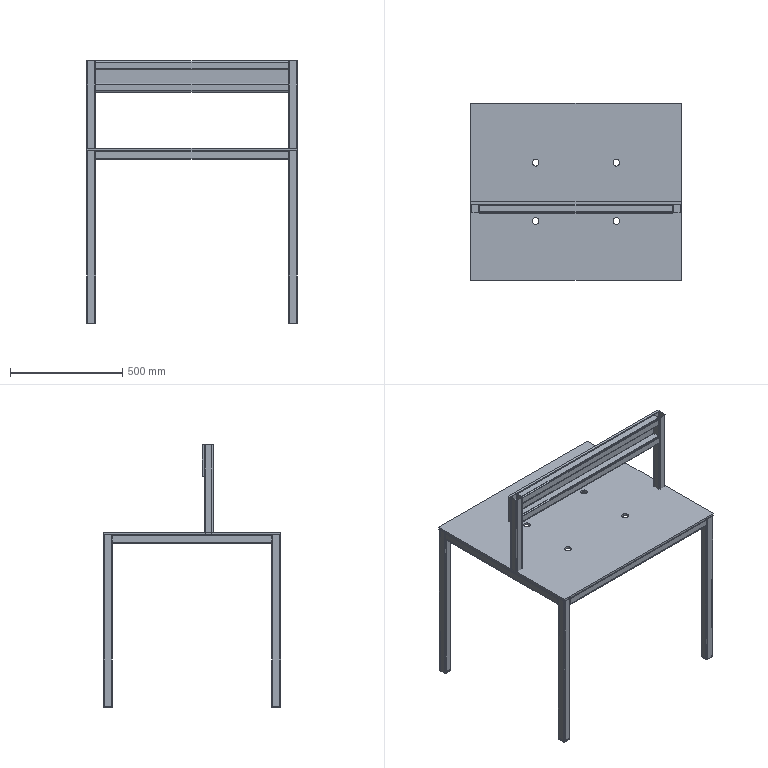Part | STEP file | MYT-A01-P32(Default_machined_) | 18 solids | 268 faces | box 940 x 790 x 1170 mm | volume 12412396 mm3 | plane 156 | cylinder 112 | commonest cylinder face diameters 6 x48 12 x48 10.2 x8 30 x8